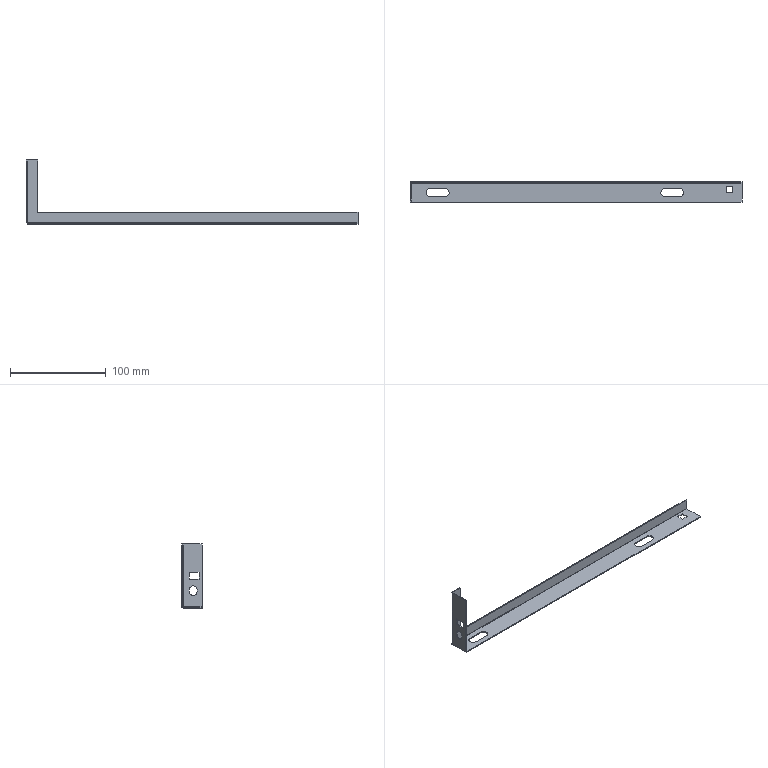Part | 1 solid | 44 faces | box 346 x 21 x 66.7 mm | volume 12385 mm3 | plane 34 | cylinder 10 | commonest cylinder face diameters 9 x4 0.4 x2 2.4 x2 8 x2
STEP:
#1=CARTESIAN_POINT('',(172.4,-1.,11.));
#2=VERTEX_POINT('',#1);
#3=CARTESIAN_POINT('',(-161.4,-1.,11.));
#4=VERTEX_POINT('',#3);
#5=CARTESIAN_POINT('',(-172.4,-1.,11.));
#6=DIRECTION('',(-1.,0.,0.));
#7=VECTOR('',#6,1000.);
#8=LINE('',#5,#7);
#9=EDGE_CURVE('',#2,#4,#8,.T.);
#10=ORIENTED_EDGE('',*,*,#9,.T.);
#11=CARTESIAN_POINT('',(-161.4,-1.,65.5));
#12=VERTEX_POINT('',#11);
#13=CARTESIAN_POINT('',(-161.4,-1.,65.5));
#14=DIRECTION('',(0.,0.,1.));
#15=VECTOR('',#14,1000.);
#16=LINE('',#13,#15);
#17=EDGE_CURVE('',#4,#12,#16,.T.);
#18=ORIENTED_EDGE('',*,*,#17,.T.);
#19=CARTESIAN_POINT('',(-172.4,-1.,65.5));
#20=VERTEX_POINT('',#19);
#21=CARTESIAN_POINT('',(-172.4,-1.,65.5));
#22=DIRECTION('',(1.,0.,0.));
#23=VECTOR('',#22,1000.);
#24=LINE('',#21,#23);
#25=EDGE_CURVE('',#20,#12,#24,.T.);
#26=ORIENTED_EDGE('',*,*,#25,.F.);
#27=CARTESIAN_POINT('',(-172.4,-1.,0.));
#28=VERTEX_POINT('',#27);
#29=CARTESIAN_POINT('',(-172.4,-1.,65.5));
#30=DIRECTION('',(0.,0.,-1.));
#31=VECTOR('',#30,1000.);
#32=LINE('',#29,#31);
#33=EDGE_CURVE('',#20,#28,#32,.T.);
#34=ORIENTED_EDGE('',*,*,#33,.T.);
#35=CARTESIAN_POINT('',(172.4,-1.,0.));
#36=VERTEX_POINT('',#35);
#37=CARTESIAN_POINT('',(-172.4,-1.,0.));
#38=DIRECTION('',(1.,0.,0.));
#39=VECTOR('',#38,1000.);
#40=LINE('',#37,#39);
#41=EDGE_CURVE('',#28,#36,#40,.T.);
#42=ORIENTED_EDGE('',*,*,#41,.T.);
#43=CARTESIAN_POINT('',(172.4,-1.,65.5));
#44=DIRECTION('',(0.,0.,-1.));
#45=VECTOR('',#44,1000.);
#46=LINE('',#43,#45);
#47=EDGE_CURVE('',#2,#36,#46,.T.);
#48=ORIENTED_EDGE('',*,*,#47,.F.);
#49=EDGE_LOOP('',(#10,#18,#26,#34,#42,#48));
#50=FACE_OUTER_BOUND('',#49,.T.);
#51=CARTESIAN_POINT('',(-172.4,-1.,65.5));
#52=DIRECTION('',(0.,1.,0.));
#53=DIRECTION('',(-1.,0.,0.));
#54=AXIS2_PLACEMENT_3D('',#51,#52,#53);
#55=PLANE('',#54);
#56=ADVANCED_FACE('',(#50),#55,.F.);
#57=CARTESIAN_POINT('',(172.4,0.,11.));
#58=VERTEX_POINT('',#57);
#59=CARTESIAN_POINT('',(172.4,-10.,11.));
#60=DIRECTION('',(0.,1.,0.));
#61=VECTOR('',#60,1000.);
#62=LINE('',#59,#61);
#63=EDGE_CURVE('',#2,#58,#62,.T.);
#64=ORIENTED_EDGE('',*,*,#63,.F.);
#65=ORIENTED_EDGE('',*,*,#47,.T.);
#66=CARTESIAN_POINT('',(172.4,0.,0.));
#67=VERTEX_POINT('',#66);
#68=CARTESIAN_POINT('',(172.4,0.,0.));
#69=DIRECTION('',(0.,-1.,0.));
#70=VECTOR('',#69,1000.);
#71=LINE('',#68,#70);
#72=EDGE_CURVE('',#67,#36,#71,.T.);
#73=ORIENTED_EDGE('',*,*,#72,.F.);
#74=CARTESIAN_POINT('',(172.4,0.,65.5));
#75=DIRECTION('',(0.,0.,-1.));
#76=VECTOR('',#75,1000.);
#77=LINE('',#74,#76);
#78=EDGE_CURVE('',#58,#67,#77,.T.);
#79=ORIENTED_EDGE('',*,*,#78,.F.);
#80=EDGE_LOOP('',(#64,#65,#73,#79));
#81=FACE_OUTER_BOUND('',#80,.T.);
#82=CARTESIAN_POINT('',(172.4,0.,65.5));
#83=DIRECTION('',(1.,0.,0.));
#84=DIRECTION('',(0.,0.,-1.));
#85=AXIS2_PLACEMENT_3D('',#82,#83,#84);
#86=PLANE('',#85);
#87=ADVANCED_FACE('',(#81),#86,.T.);
#88=CARTESIAN_POINT('',(-161.4,0.,11.));
#89=VERTEX_POINT('',#88);
#90=CARTESIAN_POINT('',(-161.4,0.,65.5));
#91=VERTEX_POINT('',#90);
#92=CARTESIAN_POINT('',(-161.4,0.,65.5));
#93=DIRECTION('',(0.,0.,1.));
#94=VECTOR('',#93,1000.);
#95=LINE('',#92,#94);
#96=EDGE_CURVE('',#89,#91,#95,.T.);
#97=ORIENTED_EDGE('',*,*,#96,.F.);
#98=CARTESIAN_POINT('',(172.4,0.,11.));
#99=DIRECTION('',(-1.,0.,0.));
#100=VECTOR('',#99,1000.);
#101=LINE('',#98,#100);
#102=EDGE_CURVE('',#58,#89,#101,.T.);
#103=ORIENTED_EDGE('',*,*,#102,.F.);
#104=ORIENTED_EDGE('',*,*,#78,.T.);
#105=CARTESIAN_POINT('',(-172.4,0.,0.));
#106=VERTEX_POINT('',#105);
#107=CARTESIAN_POINT('',(-172.4,0.,0.));
#108=DIRECTION('',(1.,0.,0.));
#109=VECTOR('',#108,1000.);
#110=LINE('',#107,#109);
#111=EDGE_CURVE('',#106,#67,#110,.T.);
#112=ORIENTED_EDGE('',*,*,#111,.F.);
#113=CARTESIAN_POINT('',(-172.4,0.,65.5));
#114=VERTEX_POINT('',#113);
#115=CARTESIAN_POINT('',(-172.4,0.,65.5));
#116=DIRECTION('',(0.,0.,-1.));
#117=VECTOR('',#116,1000.);
#118=LINE('',#115,#117);
#119=EDGE_CURVE('',#114,#106,#118,.T.);
#120=ORIENTED_EDGE('',*,*,#119,.F.);
#121=CARTESIAN_POINT('',(-172.4,0.,65.5));
#122=DIRECTION('',(1.,0.,0.));
#123=VECTOR('',#122,1000.);
#124=LINE('',#121,#123);
#125=EDGE_CURVE('',#114,#91,#124,.T.);
#126=ORIENTED_EDGE('',*,*,#125,.T.);
#127=EDGE_LOOP('',(#97,#103,#104,#112,#120,#126));
#128=FACE_OUTER_BOUND('',#127,.T.);
#129=CARTESIAN_POINT('',(-172.4,0.,65.5));
#130=DIRECTION('',(0.,1.,0.));
#131=DIRECTION('',(-1.,0.,0.));
#132=AXIS2_PLACEMENT_3D('',#129,#130,#131);
#133=PLANE('',#132);
#134=ADVANCED_FACE('',(#128),#133,.T.);
#135=ORIENTED_EDGE('',*,*,#25,.T.);
#136=CARTESIAN_POINT('',(-161.4,0.,65.5));
#137=DIRECTION('',(0.,1.,0.));
#138=VECTOR('',#137,1000.);
#139=LINE('',#136,#138);
#140=EDGE_CURVE('',#12,#91,#139,.T.);
#141=ORIENTED_EDGE('',*,*,#140,.T.);
#142=ORIENTED_EDGE('',*,*,#125,.F.);
#143=CARTESIAN_POINT('',(-172.4,-1.,65.5));
#144=DIRECTION('',(0.,1.,0.));
#145=VECTOR('',#144,1000.);
#146=LINE('',#143,#145);
#147=EDGE_CURVE('',#20,#114,#146,.T.);
#148=ORIENTED_EDGE('',*,*,#147,.F.);
#149=EDGE_LOOP('',(#135,#141,#142,#148));
#150=FACE_OUTER_BOUND('',#149,.T.);
#151=CARTESIAN_POINT('',(0.,0.,65.5));
#152=DIRECTION('',(0.,0.,-1.));
#153=DIRECTION('',(-1.,0.,0.));
#154=AXIS2_PLACEMENT_3D('',#151,#152,#153);
#155=PLANE('',#154);
#156=ADVANCED_FACE('',(#150),#155,.F.);
#157=ORIENTED_EDGE('',*,*,#63,.T.);
#158=ORIENTED_EDGE('',*,*,#102,.T.);
#159=CARTESIAN_POINT('',(-161.4,-10.,11.));
#160=DIRECTION('',(0.,1.,0.));
#161=VECTOR('',#160,1000.);
#162=LINE('',#159,#161);
#163=EDGE_CURVE('',#4,#89,#162,.T.);
#164=ORIENTED_EDGE('',*,*,#163,.F.);
#165=ORIENTED_EDGE('',*,*,#9,.F.);
#166=EDGE_LOOP('',(#157,#158,#164,#165));
#167=FACE_OUTER_BOUND('',#166,.T.);
#168=CARTESIAN_POINT('',(172.4,-10.,11.));
#169=DIRECTION('',(0.,0.,-1.));
#170=DIRECTION('',(-1.,0.,0.));
#171=AXIS2_PLACEMENT_3D('',#168,#169,#170);
#172=PLANE('',#171);
#173=ADVANCED_FACE('',(#167),#172,.F.);
#174=ORIENTED_EDGE('',*,*,#163,.T.);
#175=ORIENTED_EDGE('',*,*,#96,.T.);
#176=ORIENTED_EDGE('',*,*,#140,.F.);
#177=ORIENTED_EDGE('',*,*,#17,.F.);
#178=EDGE_LOOP('',(#174,#175,#176,#177));
#179=FACE_OUTER_BOUND('',#178,.T.);
#180=CARTESIAN_POINT('',(-161.4,-10.,65.5));
#181=DIRECTION('',(-1.,0.,0.));
#182=DIRECTION('',(0.,0.,1.));
#183=AXIS2_PLACEMENT_3D('',#180,#181,#182);
#184=PLANE('',#183);
#185=ADVANCED_FACE('',(#179),#184,.F.);
#186=CARTESIAN_POINT('',(-172.4,-1.2,-0.2));
#187=VERTEX_POINT('',#186);
#188=CARTESIAN_POINT('',(-172.4,-1.2,-1.2));
#189=VERTEX_POINT('',#188);
#190=CARTESIAN_POINT('',(-172.4,-1.2,-1.2));
#191=DIRECTION('',(0.,0.,-1.));
#192=VECTOR('',#191,1000.);
#193=LINE('',#190,#192);
#194=EDGE_CURVE('',#187,#189,#193,.T.);
#195=ORIENTED_EDGE('',*,*,#194,.F.);
#196=CARTESIAN_POINT('',(-172.4,-1.2,0.));
#197=DIRECTION('',(-1.,0.,0.));
#198=DIRECTION('',(0.,1.,0.));
#199=AXIS2_PLACEMENT_3D('',#196,#197,#198);
#200=CIRCLE('',#199,0.2);
#201=EDGE_CURVE('',#28,#187,#200,.T.);
#202=ORIENTED_EDGE('',*,*,#201,.F.);
#203=CARTESIAN_POINT('',(-172.4,-1.,0.));
#204=DIRECTION('',(0.,1.,0.));
#205=VECTOR('',#204,1000.);
#206=LINE('',#203,#205);
#207=EDGE_CURVE('',#28,#106,#206,.T.);
#208=ORIENTED_EDGE('',*,*,#207,.T.);
#209=CARTESIAN_POINT('',(-172.4,-1.2,0.));
#210=DIRECTION('',(-1.,0.,0.));
#211=DIRECTION('',(0.,1.,0.));
#212=AXIS2_PLACEMENT_3D('',#209,#210,#211);
#213=CIRCLE('',#212,1.2);
#214=EDGE_CURVE('',#106,#189,#213,.T.);
#215=ORIENTED_EDGE('',*,*,#214,.T.);
#216=EDGE_LOOP('',(#195,#202,#208,#215));
#217=FACE_OUTER_BOUND('',#216,.T.);
#218=CARTESIAN_POINT('',(-172.4,-1.2,0.));
#219=DIRECTION('',(-1.,0.,0.));
#220=DIRECTION('',(0.,-1.,0.));
#221=AXIS2_PLACEMENT_3D('',#218,#219,#220);
#222=PLANE('',#221);
#223=ADVANCED_FACE('',(#217),#222,.T.);
#224=CARTESIAN_POINT('',(172.4,-1.2,-0.2));
#225=VERTEX_POINT('',#224);
#226=CARTESIAN_POINT('',(172.4,-1.2,0.));
#227=DIRECTION('',(1.,0.,0.));
#228=DIRECTION('',(0.,1.,0.));
#229=AXIS2_PLACEMENT_3D('',#226,#227,#228);
#230=CIRCLE('',#229,0.2);
#231=EDGE_CURVE('',#225,#36,#230,.T.);
#232=ORIENTED_EDGE('',*,*,#231,.F.);
#233=CARTESIAN_POINT('',(172.4,-1.2,-1.2));
#234=VERTEX_POINT('',#233);
#235=CARTESIAN_POINT('',(172.4,-1.2,-0.2));
#236=DIRECTION('',(0.,0.,-1.));
#237=VECTOR('',#236,1000.);
#238=LINE('',#235,#237);
#239=EDGE_CURVE('',#225,#234,#238,.T.);
#240=ORIENTED_EDGE('',*,*,#239,.T.);
#241=CARTESIAN_POINT('',(172.4,-1.2,0.));
#242=DIRECTION('',(1.,0.,0.));
#243=DIRECTION('',(0.,1.,0.));
#244=AXIS2_PLACEMENT_3D('',#241,#242,#243);
#245=CIRCLE('',#244,1.2);
#246=EDGE_CURVE('',#234,#67,#245,.T.);
#247=ORIENTED_EDGE('',*,*,#246,.T.);
#248=ORIENTED_EDGE('',*,*,#72,.T.);
#249=EDGE_LOOP('',(#232,#240,#247,#248));
#250=FACE_OUTER_BOUND('',#249,.T.);
#251=CARTESIAN_POINT('',(172.4,-1.2,0.));
#252=DIRECTION('',(-1.,0.,0.));
#253=DIRECTION('',(0.,-1.,0.));
#254=AXIS2_PLACEMENT_3D('',#251,#252,#253);
#255=PLANE('',#254);
#256=ADVANCED_FACE('',(#250),#255,.F.);
#257=ORIENTED_EDGE('',*,*,#111,.T.);
#258=ORIENTED_EDGE('',*,*,#246,.F.);
#259=CARTESIAN_POINT('',(0.,-1.2,-1.2));
#260=DIRECTION('',(1.,0.,0.));
#261=VECTOR('',#260,1000.);
#262=LINE('',#259,#261);
#263=EDGE_CURVE('',#189,#234,#262,.T.);
#264=ORIENTED_EDGE('',*,*,#263,.F.);
#265=ORIENTED_EDGE('',*,*,#214,.F.);
#266=EDGE_LOOP('',(#257,#258,#264,#265));
#267=FACE_OUTER_BOUND('',#266,.T.);
#268=CARTESIAN_POINT('',(172.4,-1.2,0.));
#269=DIRECTION('',(1.,0.,0.));
#270=DIRECTION('',(0.,0.,-1.));
#271=AXIS2_PLACEMENT_3D('',#268,#269,#270);
#272=CYLINDRICAL_SURFACE('',#271,1.2);
#273=ADVANCED_FACE('',(#267),#272,.T.);
#274=ORIENTED_EDGE('',*,*,#41,.F.);
#275=ORIENTED_EDGE('',*,*,#201,.T.);
#276=CARTESIAN_POINT('',(-172.4,-1.2,-0.2));
#277=DIRECTION('',(1.,0.,0.));
#278=VECTOR('',#277,1000.);
#279=LINE('',#276,#278);
#280=EDGE_CURVE('',#187,#225,#279,.T.);
#281=ORIENTED_EDGE('',*,*,#280,.T.);
#282=ORIENTED_EDGE('',*,*,#231,.T.);
#283=EDGE_LOOP('',(#274,#275,#281,#282));
#284=FACE_OUTER_BOUND('',#283,.T.);
#285=CARTESIAN_POINT('',(172.4,-1.2,0.));
#286=DIRECTION('',(1.,0.,0.));
#287=DIRECTION('',(0.,0.,-1.));
#288=AXIS2_PLACEMENT_3D('',#285,#286,#287);
#289=CYLINDRICAL_SURFACE('',#288,0.2);
#290=ADVANCED_FACE('',(#284),#289,.F.);
#291=CARTESIAN_POINT('',(172.4,-21.,-1.2));
#292=VERTEX_POINT('',#291);
#293=CARTESIAN_POINT('',(172.4,-1.,-1.2));
#294=DIRECTION('',(0.,1.,0.));
#295=VECTOR('',#294,1000.);
#296=LINE('',#293,#295);
#297=EDGE_CURVE('',#292,#234,#296,.T.);
#298=ORIENTED_EDGE('',*,*,#297,.T.);
#299=ORIENTED_EDGE('',*,*,#239,.F.);
#300=CARTESIAN_POINT('',(172.4,-21.,-0.2));
#301=VERTEX_POINT('',#300);
#302=CARTESIAN_POINT('',(172.4,0.,-0.2));
#303=DIRECTION('',(0.,1.,0.));
#304=VECTOR('',#303,1000.);
#305=LINE('',#302,#304);
#306=EDGE_CURVE('',#301,#225,#305,.T.);
#307=ORIENTED_EDGE('',*,*,#306,.F.);
#308=CARTESIAN_POINT('',(172.4,-21.,-1.2));
#309=DIRECTION('',(0.,0.,1.));
#310=VECTOR('',#309,1000.);
#311=LINE('',#308,#310);
#312=EDGE_CURVE('',#292,#301,#311,.T.);
#313=ORIENTED_EDGE('',*,*,#312,.F.);
#314=EDGE_LOOP('',(#298,#299,#307,#313));
#315=FACE_OUTER_BOUND('',#314,.T.);
#316=CARTESIAN_POINT('',(172.4,-1.,-1.2));
#317=DIRECTION('',(1.,0.,0.));
#318=DIRECTION('',(0.,0.,-1.));
#319=AXIS2_PLACEMENT_3D('',#316,#317,#318);
#320=PLANE('',#319);
#321=ADVANCED_FACE('',(#315),#320,.T.);
#322=CARTESIAN_POINT('',(-172.4,-21.,-0.2));
#323=VERTEX_POINT('',#322);
#324=CARTESIAN_POINT('',(-172.4,0.,-0.2));
#325=DIRECTION('',(0.,-1.,0.));
#326=VECTOR('',#325,1000.);
#327=LINE('',#324,#326);
#328=EDGE_CURVE('',#187,#323,#327,.T.);
#329=ORIENTED_EDGE('',*,*,#328,.F.);
#330=ORIENTED_EDGE('',*,*,#194,.T.);
#331=CARTESIAN_POINT('',(-172.4,-21.,-1.2));
#332=VERTEX_POINT('',#331);
#333=CARTESIAN_POINT('',(-172.4,-21.,-1.2));
#334=DIRECTION('',(0.,-1.,0.));
#335=VECTOR('',#334,1000.);
#336=LINE('',#333,#335);
#337=EDGE_CURVE('',#189,#332,#336,.T.);
#338=ORIENTED_EDGE('',*,*,#337,.T.);
#339=CARTESIAN_POINT('',(-172.4,-21.,-1.2));
#340=DIRECTION('',(0.,0.,1.));
#341=VECTOR('',#340,1000.);
#342=LINE('',#339,#341);
#343=EDGE_CURVE('',#332,#323,#342,.T.);
#344=ORIENTED_EDGE('',*,*,#343,.T.);
#345=EDGE_LOOP('',(#329,#330,#338,#344));
#346=FACE_OUTER_BOUND('',#345,.T.);
#347=CARTESIAN_POINT('',(-172.4,-21.,-1.2));
#348=DIRECTION('',(-1.,0.,0.));
#349=DIRECTION('',(0.,0.,1.));
#350=AXIS2_PLACEMENT_3D('',#347,#348,#349);
#351=PLANE('',#350);
#352=ADVANCED_FACE('',(#346),#351,.T.);
#353=CARTESIAN_POINT('',(162.9,-4.3,-1.2));
#354=VERTEX_POINT('',#353);
#355=CARTESIAN_POINT('',(162.9,-11.3,-1.2));
#356=VERTEX_POINT('',#355);
#357=CARTESIAN_POINT('',(162.9,-11.3,-1.2));
#358=DIRECTION('',(0.,-1.,0.));
#359=VECTOR('',#358,1000.);
#360=LINE('',#357,#359);
#361=EDGE_CURVE('',#354,#356,#360,.T.);
#362=ORIENTED_EDGE('',*,*,#361,.F.);
#363=CARTESIAN_POINT('',(155.9,-4.3,-1.2));
#364=VERTEX_POINT('',#363);
#365=CARTESIAN_POINT('',(162.9,-4.3,-1.2));
#366=DIRECTION('',(1.,0.,0.));
#367=VECTOR('',#366,1000.);
#368=LINE('',#365,#367);
#369=EDGE_CURVE('',#364,#354,#368,.T.);
#370=ORIENTED_EDGE('',*,*,#369,.F.);
#371=CARTESIAN_POINT('',(155.9,-11.3,-1.2));
#372=VERTEX_POINT('',#371);
#373=CARTESIAN_POINT('',(155.9,-11.3,-1.2));
#374=DIRECTION('',(0.,1.,0.));
#375=VECTOR('',#374,1000.);
#376=LINE('',#373,#375);
#377=EDGE_CURVE('',#372,#364,#376,.T.);
#378=ORIENTED_EDGE('',*,*,#377,.F.);
#379=CARTESIAN_POINT('',(162.9,-11.3,-1.2));
#380=DIRECTION('',(-1.,0.,0.));
#381=VECTOR('',#380,1000.);
#382=LINE('',#379,#381);
#383=EDGE_CURVE('',#356,#372,#382,.T.);
#384=ORIENTED_EDGE('',*,*,#383,.F.);
#385=EDGE_LOOP('',(#362,#370,#378,#384));
#386=FACE_BOUND('',#385,.T.);
#387=CARTESIAN_POINT('',(-152.3,-15.5,-1.2));
#388=VERTEX_POINT('',#387);
#389=CARTESIAN_POINT('',(-152.3,-6.5,-1.2));
#390=VERTEX_POINT('',#389);
#391=CARTESIAN_POINT('',(-152.3,-11.,-1.2));
#392=DIRECTION('',(0.,0.,-1.));
#393=DIRECTION('',(0.,1.,0.));
#394=AXIS2_PLACEMENT_3D('',#391,#392,#393);
#395=CIRCLE('',#394,4.5);
#396=EDGE_CURVE('',#388,#390,#395,.T.);
#397=ORIENTED_EDGE('',*,*,#396,.F.);
#398=CARTESIAN_POINT('',(-137.3,-15.5,-1.2));
#399=VERTEX_POINT('',#398);
#400=CARTESIAN_POINT('',(-152.3,-15.5,-1.2));
#401=DIRECTION('',(-1.,0.,0.));
#402=VECTOR('',#401,1000.);
#403=LINE('',#400,#402);
#404=EDGE_CURVE('',#399,#388,#403,.T.);
#405=ORIENTED_EDGE('',*,*,#404,.F.);
#406=CARTESIAN_POINT('',(-137.3,-6.5,-1.2));
#407=VERTEX_POINT('',#406);
#408=CARTESIAN_POINT('',(-137.3,-11.,-1.2));
#409=DIRECTION('',(0.,0.,-1.));
#410=DIRECTION('',(0.,1.,0.));
#411=AXIS2_PLACEMENT_3D('',#408,#409,#410);
#412=CIRCLE('',#411,4.5);
#413=EDGE_CURVE('',#407,#399,#412,.T.);
#414=ORIENTED_EDGE('',*,*,#413,.F.);
#415=CARTESIAN_POINT('',(-152.3,-6.5,-1.2));
#416=DIRECTION('',(1.,0.,0.));
#417=VECTOR('',#416,1000.);
#418=LINE('',#415,#417);
#419=EDGE_CURVE('',#390,#407,#418,.T.);
#420=ORIENTED_EDGE('',*,*,#419,.F.);
#421=EDGE_LOOP('',(#397,#405,#414,#420));
#422=FACE_BOUND('',#421,.T.);
#423=CARTESIAN_POINT('',(92.2,-15.5,-1.2));
#424=VERTEX_POINT('',#423);
#425=CARTESIAN_POINT('',(92.2,-6.5,-1.2));
#426=VERTEX_POINT('',#425);
#427=CARTESIAN_POINT('',(92.2,-11.,-1.2));
#428=DIRECTION('',(0.,0.,-1.));
#429=DIRECTION('',(0.,1.,0.));
#430=AXIS2_PLACEMENT_3D('',#427,#428,#429);
#431=CIRCLE('',#430,4.5);
#432=EDGE_CURVE('',#424,#426,#431,.T.);
#433=ORIENTED_EDGE('',*,*,#432,.F.);
#434=CARTESIAN_POINT('',(107.2,-15.5,-1.2));
#435=VERTEX_POINT('',#434);
#436=CARTESIAN_POINT('',(92.2,-15.5,-1.2));
#437=DIRECTION('',(-1.,0.,0.));
#438=VECTOR('',#437,1000.);
#439=LINE('',#436,#438);
#440=EDGE_CURVE('',#435,#424,#439,.T.);
#441=ORIENTED_EDGE('',*,*,#440,.F.);
#442=CARTESIAN_POINT('',(107.2,-6.5,-1.2));
#443=VERTEX_POINT('',#442);
#444=CARTESIAN_POINT('',(107.2,-11.,-1.2));
#445=DIRECTION('',(0.,0.,-1.));
#446=DIRECTION('',(0.,1.,0.));
#447=AXIS2_PLACEMENT_3D('',#444,#445,#446);
#448=CIRCLE('',#447,4.5);
#449=EDGE_CURVE('',#443,#435,#448,.T.);
#450=ORIENTED_EDGE('',*,*,#449,.F.);
#451=CARTESIAN_POINT('',(92.2,-6.5,-1.2));
#452=DIRECTION('',(1.,0.,0.));
#453=VECTOR('',#452,1000.);
#454=LINE('',#451,#453);
#455=EDGE_CURVE('',#426,#443,#454,.T.);
#456=ORIENTED_EDGE('',*,*,#455,.F.);
#457=EDGE_LOOP('',(#433,#441,#450,#456));
#458=FACE_BOUND('',#457,.T.);
#459=ORIENTED_EDGE('',*,*,#337,.F.);
#460=ORIENTED_EDGE('',*,*,#263,.T.);
#461=ORIENTED_EDGE('',*,*,#297,.F.);
#462=CARTESIAN_POINT('',(172.4,-21.,-1.2));
#463=DIRECTION('',(1.,0.,0.));
#464=VECTOR('',#463,1000.);
#465=LINE('',#462,#464);
#466=EDGE_CURVE('',#332,#292,#465,.T.);
#467=ORIENTED_EDGE('',*,*,#466,.F.);
#468=EDGE_LOOP('',(#459,#460,#461,#467));
#469=FACE_OUTER_BOUND('',#468,.T.);
#470=CARTESIAN_POINT('',(0.,0.,-1.2));
#471=DIRECTION('',(0.,0.,-1.));
#472=DIRECTION('',(0.,1.,0.));
#473=AXIS2_PLACEMENT_3D('',#470,#471,#472);
#474=PLANE('',#473);
#475=ADVANCED_FACE('',(#386,#422,#458,#469),#474,.T.);
#476=CARTESIAN_POINT('',(155.9,-4.3,-0.2));
#477=VERTEX_POINT('',#476);
#478=CARTESIAN_POINT('',(162.9,-4.3,-0.2));
#479=VERTEX_POINT('',#478);
#480=CARTESIAN_POINT('',(0.,-4.3,-0.2));
#481=DIRECTION('',(1.,0.,0.));
#482=VECTOR('',#481,1000.);
#483=LINE('',#480,#482);
#484=EDGE_CURVE('',#477,#479,#483,.T.);
#485=ORIENTED_EDGE('',*,*,#484,.T.);
#486=CARTESIAN_POINT('',(162.9,-11.3,-0.2));
#487=VERTEX_POINT('',#486);
#488=CARTESIAN_POINT('',(162.9,0.,-0.2));
#489=DIRECTION('',(0.,-1.,0.));
#490=VECTOR('',#489,1000.);
#491=LINE('',#488,#490);
#492=EDGE_CURVE('',#479,#487,#491,.T.);
#493=ORIENTED_EDGE('',*,*,#492,.T.);
#494=CARTESIAN_POINT('',(155.9,-11.3,-0.2));
#495=VERTEX_POINT('',#494);
#496=CARTESIAN_POINT('',(0.,-11.3,-0.2));
#497=DIRECTION('',(-1.,0.,0.));
#498=VECTOR('',#497,1000.);
#499=LINE('',#496,#498);
#500=EDGE_CURVE('',#487,#495,#499,.T.);
#501=ORIENTED_EDGE('',*,*,#500,.T.);
#502=CARTESIAN_POINT('',(155.9,0.,-0.2));
#503=DIRECTION('',(0.,1.,0.));
#504=VECTOR('',#503,1000.);
#505=LINE('',#502,#504);
#506=EDGE_CURVE('',#495,#477,#505,.T.);
#507=ORIENTED_EDGE('',*,*,#506,.T.);
#508=EDGE_LOOP('',(#485,#493,#501,#507));
#509=FACE_BOUND('',#508,.T.);
#510=CARTESIAN_POINT('',(-137.3,-15.5,-0.2));
#511=VERTEX_POINT('',#510);
#512=CARTESIAN_POINT('',(-152.3,-15.5,-0.2));
#513=VERTEX_POINT('',#512);
#514=CARTESIAN_POINT('',(0.,-15.5,-0.2));
#515=DIRECTION('',(-1.,0.,0.));
#516=VECTOR('',#515,1000.);
#517=LINE('',#514,#516);
#518=EDGE_CURVE('',#511,#513,#517,.T.);
#519=ORIENTED_EDGE('',*,*,#518,.T.);
#520=CARTESIAN_POINT('',(-152.3,-6.5,-0.2));
#521=VERTEX_POINT('',#520);
#522=CARTESIAN_POINT('',(-152.3,-11.,-0.2));
#523=DIRECTION('',(0.,0.,-1.));
#524=DIRECTION('',(0.,1.,0.));
#525=AXIS2_PLACEMENT_3D('',#522,#523,#524);
#526=CIRCLE('',#525,4.5);
#527=EDGE_CURVE('',#513,#521,#526,.T.);
#528=ORIENTED_EDGE('',*,*,#527,.T.);
#529=CARTESIAN_POINT('',(-137.3,-6.5,-0.2));
#530=VERTEX_POINT('',#529);
#531=CARTESIAN_POINT('',(0.,-6.5,-0.2));
#532=DIRECTION('',(1.,0.,0.));
#533=VECTOR('',#532,1000.);
#534=LINE('',#531,#533);
#535=EDGE_CURVE('',#521,#530,#534,.T.);
#536=ORIENTED_EDGE('',*,*,#535,.T.);
#537=CARTESIAN_POINT('',(-137.3,-11.,-0.2));
#538=DIRECTION('',(0.,0.,-1.));
#539=DIRECTION('',(0.,1.,0.));
#540=AXIS2_PLACEMENT_3D('',#537,#538,#539);
#541=CIRCLE('',#540,4.5);
#542=EDGE_CURVE('',#530,#511,#541,.T.);
#543=ORIENTED_EDGE('',*,*,#542,.T.);
#544=EDGE_LOOP('',(#519,#528,#536,#543));
#545=FACE_BOUND('',#544,.T.);
#546=CARTESIAN_POINT('',(107.2,-15.5,-0.2));
#547=VERTEX_POINT('',#546);
#548=CARTESIAN_POINT('',(92.2,-15.5,-0.2));
#549=VERTEX_POINT('',#548);
#550=CARTESIAN_POINT('',(0.,-15.5,-0.2));
#551=DIRECTION('',(-1.,0.,0.));
#552=VECTOR('',#551,1000.);
#553=LINE('',#550,#552);
#554=EDGE_CURVE('',#547,#549,#553,.T.);
#555=ORIENTED_EDGE('',*,*,#554,.T.);
#556=CARTESIAN_POINT('',(92.2,-6.5,-0.2));
#557=VERTEX_POINT('',#556);
#558=CARTESIAN_POINT('',(92.2,-11.,-0.2));
#559=DIRECTION('',(0.,0.,-1.));
#560=DIRECTION('',(0.,1.,0.));
#561=AXIS2_PLACEMENT_3D('',#558,#559,#560);
#562=CIRCLE('',#561,4.5);
#563=EDGE_CURVE('',#549,#557,#562,.T.);
#564=ORIENTED_EDGE('',*,*,#563,.T.);
#565=CARTESIAN_POINT('',(107.2,-6.5,-0.2));
#566=VERTEX_POINT('',#565);
#567=CARTESIAN_POINT('',(0.,-6.5,-0.2));
#568=DIRECTION('',(1.,0.,0.));
#569=VECTOR('',#568,1000.);
#570=LINE('',#567,#569);
#571=EDGE_CURVE('',#557,#566,#570,.T.);
#572=ORIENTED_EDGE('',*,*,#571,.T.);
#573=CARTESIAN_POINT('',(107.2,-11.,-0.2));
#574=DIRECTION('',(0.,0.,-1.));
#575=DIRECTION('',(0.,1.,0.));
#576=AXIS2_PLACEMENT_3D('',#573,#574,#575);
#577=CIRCLE('',#576,4.5);
#578=EDGE_CURVE('',#566,#547,#577,.T.);
#579=ORIENTED_EDGE('',*,*,#578,.T.);
#580=EDGE_LOOP('',(#555,#564,#572,#579));
#581=FACE_BOUND('',#580,.T.);
#582=ORIENTED_EDGE('',*,*,#280,.F.);
#583=ORIENTED_EDGE('',*,*,#328,.T.);
#584=CARTESIAN_POINT('',(0.,-21.,-0.2));
#585=DIRECTION('',(1.,0.,0.));
#586=VECTOR('',#585,1000.);
#587=LINE('',#584,#586);
#588=EDGE_CURVE('',#323,#301,#587,.T.);
#589=ORIENTED_EDGE('',*,*,#588,.T.);
#590=ORIENTED_EDGE('',*,*,#306,.T.);
#591=EDGE_LOOP('',(#582,#583,#589,#590));
#592=FACE_OUTER_BOUND('',#591,.T.);
#593=CARTESIAN_POINT('',(0.,0.,-0.2));
#594=DIRECTION('',(0.,0.,-1.));
#595=DIRECTION('',(0.,1.,0.));
#596=AXIS2_PLACEMENT_3D('',#593,#594,#595);
#597=PLANE('',#596);
#598=ADVANCED_FACE('',(#509,#545,#581,#592),#597,.F.);
#599=ORIENTED_EDGE('',*,*,#588,.F.);
#600=ORIENTED_EDGE('',*,*,#343,.F.);
#601=ORIENTED_EDGE('',*,*,#466,.T.);
#602=ORIENTED_EDGE('',*,*,#312,.T.);
#603=EDGE_LOOP('',(#599,#600,#601,#602));
#604=FACE_OUTER_BOUND('',#603,.T.);
#605=CARTESIAN_POINT('',(172.4,-21.,-1.2));
#606=DIRECTION('',(0.,-1.,0.));
#607=DIRECTION('',(0.,0.,-1.));
#608=AXIS2_PLACEMENT_3D('',#605,#606,#607);
#609=PLANE('',#608);
#610=ADVANCED_FACE('',(#604),#609,.T.);
#611=CARTESIAN_POINT('',(-172.6,-1.2,65.5));
#612=VERTEX_POINT('',#611);
#613=CARTESIAN_POINT('',(-173.6,-1.2,65.5));
#614=VERTEX_POINT('',#613);
#615=CARTESIAN_POINT('',(-173.6,-1.2,65.5));
#616=DIRECTION('',(-1.,0.,0.));
#617=VECTOR('',#616,1000.);
#618=LINE('',#615,#617);
#619=EDGE_CURVE('',#612,#614,#618,.T.);
#620=ORIENTED_EDGE('',*,*,#619,.F.);
#621=CARTESIAN_POINT('',(-172.4,-1.2,65.5));
#622=DIRECTION('',(0.,0.,1.));
#623=DIRECTION('',(-1.,0.,0.));
#624=AXIS2_PLACEMENT_3D('',#621,#622,#623);
#625=CIRCLE('',#624,0.2);
#626=EDGE_CURVE('',#20,#612,#625,.T.);
#627=ORIENTED_EDGE('',*,*,#626,.F.);
#628=ORIENTED_EDGE('',*,*,#147,.T.);
#629=CARTESIAN_POINT('',(-172.4,-1.2,65.5));
#630=DIRECTION('',(0.,0.,1.));
#631=DIRECTION('',(-1.,0.,0.));
#632=AXIS2_PLACEMENT_3D('',#629,#630,#631);
#633=CIRCLE('',#632,1.2);
#634=EDGE_CURVE('',#114,#614,#633,.T.);
#635=ORIENTED_EDGE('',*,*,#634,.T.);
#636=EDGE_LOOP('',(#620,#627,#628,#635));
#637=FACE_OUTER_BOUND('',#636,.T.);
#638=CARTESIAN_POINT('',(-172.4,-1.2,65.5));
#639=DIRECTION('',(0.,0.,1.));
#640=DIRECTION('',(1.,0.,0.));
#641=AXIS2_PLACEMENT_3D('',#638,#639,#640);
#642=PLANE('',#641);
#643=ADVANCED_FACE('',(#637),#642,.T.);
#644=CARTESIAN_POINT('',(-172.6,-1.2,0.));
#645=VERTEX_POINT('',#644);
#646=CARTESIAN_POINT('',(-172.4,-1.2,0.));
#647=DIRECTION('',(0.,0.,-1.));
#648=DIRECTION('',(-1.,0.,0.));
#649=AXIS2_PLACEMENT_3D('',#646,#647,#648);
#650=CIRCLE('',#649,0.2);
#651=EDGE_CURVE('',#645,#28,#650,.T.);
#652=ORIENTED_EDGE('',*,*,#651,.F.);
#653=CARTESIAN_POINT('',(-173.6,-1.2,0.));
#654=VERTEX_POINT('',#653);
#655=CARTESIAN_POINT('',(-172.6,-1.2,0.));
#656=DIRECTION('',(-1.,0.,0.));
#657=VECTOR('',#656,1000.);
#658=LINE('',#655,#657);
#659=EDGE_CURVE('',#645,#654,#658,.T.);
#660=ORIENTED_EDGE('',*,*,#659,.T.);
#661=CARTESIAN_POINT('',(-172.4,-1.2,0.));
#662=DIRECTION('',(0.,0.,-1.));
#663=DIRECTION('',(-1.,0.,0.));
#664=AXIS2_PLACEMENT_3D('',#661,#662,#663);
#665=CIRCLE('',#664,1.2);
#666=EDGE_CURVE('',#654,#106,#665,.T.);
#667=ORIENTED_EDGE('',*,*,#666,.T.);
#668=ORIENTED_EDGE('',*,*,#207,.F.);
#669=EDGE_LOOP('',(#652,#660,#667,#668));
#670=FACE_OUTER_BOUND('',#669,.T.);
#671=CARTESIAN_POINT('',(-172.4,-1.2,0.));
#672=DIRECTION('',(0.,0.,1.));
#673=DIRECTION('',(1.,0.,0.));
#674=AXIS2_PLACEMENT_3D('',#671,#672,#673);
#675=PLANE('',#674);
#676=ADVANCED_FACE('',(#670),#675,.F.);
#677=ORIENTED_EDGE('',*,*,#119,.T.);
#678=ORIENTED_EDGE('',*,*,#666,.F.);
#679=CARTESIAN_POINT('',(-173.6,-1.2,0.));
#680=DIRECTION('',(0.,0.,-1.));
#681=VECTOR('',#680,1000.);
#682=LINE('',#679,#681);
#683=EDGE_CURVE('',#614,#654,#682,.T.);
#684=ORIENTED_EDGE('',*,*,#683,.F.);
#685=ORIENTED_EDGE('',*,*,#634,.F.);
#686=EDGE_LOOP('',(#677,#678,#684,#685));
#687=FACE_OUTER_BOUND('',#686,.T.);
#688=CARTESIAN_POINT('',(-172.4,-1.2,0.));
#689=DIRECTION('',(0.,0.,-1.));
#690=DIRECTION('',(-1.,0.,0.));
#691=AXIS2_PLACEMENT_3D('',#688,#689,#690);
#692=CYLINDRICAL_SURFACE('',#691,1.2);
#693=ADVANCED_FACE('',(#687),#692,.T.);
#694=ORIENTED_EDGE('',*,*,#33,.F.);
#695=ORIENTED_EDGE('',*,*,#626,.T.);
#696=CARTESIAN_POINT('',(-172.6,-1.2,65.5));
#697=DIRECTION('',(0.,0.,-1.));
#698=VECTOR('',#697,1000.);
#699=LINE('',#696,#698);
#700=EDGE_CURVE('',#612,#645,#699,.T.);
#701=ORIENTED_EDGE('',*,*,#700,.T.);
#702=ORIENTED_EDGE('',*,*,#651,.T.);
#703=EDGE_LOOP('',(#694,#695,#701,#702));
#704=FACE_OUTER_BOUND('',#703,.T.);
#705=CARTESIAN_POINT('',(-172.4,-1.2,0.));
#706=DIRECTION('',(0.,0.,-1.));
#707=DIRECTION('',(-1.,0.,0.));
#708=AXIS2_PLACEMENT_3D('',#705,#706,#707);
#709=CYLINDRICAL_SURFACE('',#708,0.2);
#710=ADVANCED_FACE('',(#704),#709,.F.);
#711=CARTESIAN_POINT('',(-173.6,-21.,0.));
#712=VERTEX_POINT('',#711);
#713=CARTESIAN_POINT('',(-173.6,-1.,0.));
#714=DIRECTION('',(0.,1.,0.));
#715=VECTOR('',#714,1000.);
#716=LINE('',#713,#715);
#717=EDGE_CURVE('',#712,#654,#716,.T.);
#718=ORIENTED_EDGE('',*,*,#717,.T.);
#719=ORIENTED_EDGE('',*,*,#659,.F.);
#720=CARTESIAN_POINT('',(-172.6,-21.,0.));
#721=VERTEX_POINT('',#720);
#722=CARTESIAN_POINT('',(-172.6,0.,0.));
#723=DIRECTION('',(0.,1.,0.));
#724=VECTOR('',#723,1000.);
#725=LINE('',#722,#724);
#726=EDGE_CURVE('',#721,#645,#725,.T.);
#727=ORIENTED_EDGE('',*,*,#726,.F.);
#728=CARTESIAN_POINT('',(-173.6,-21.,0.));
#729=DIRECTION('',(1.,0.,0.));
#730=VECTOR('',#729,1000.);
#731=LINE('',#728,#730);
#732=EDGE_CURVE('',#712,#721,#731,.T.);
#733=ORIENTED_EDGE('',*,*,#732,.F.);
#734=EDGE_LOOP('',(#718,#719,#727,#733));
#735=FACE_OUTER_BOUND('',#734,.T.);
#736=CARTESIAN_POINT('',(-173.6,-1.,0.));
#737=DIRECTION('',(0.,0.,-1.));
#738=DIRECTION('',(-1.,0.,0.));
#739=AXIS2_PLACEMENT_3D('',#736,#737,#738);
#740=PLANE('',#739);
#741=ADVANCED_FACE('',(#735),#740,.T.);
#742=CARTESIAN_POINT('',(-172.6,-21.,65.5));
#743=VERTEX_POINT('',#742);
#744=CARTESIAN_POINT('',(-172.6,0.,65.5));
#745=DIRECTION('',(0.,-1.,0.));
#746=VECTOR('',#745,1000.);
#747=LINE('',#744,#746);
#748=EDGE_CURVE('',#612,#743,#747,.T.);
#749=ORIENTED_EDGE('',*,*,#748,.F.);
#750=ORIENTED_EDGE('',*,*,#619,.T.);
#751=CARTESIAN_POINT('',(-173.6,-21.,65.5));
#752=VERTEX_POINT('',#751);
#753=CARTESIAN_POINT('',(-173.6,-21.,65.5));
#754=DIRECTION('',(0.,-1.,0.));
#755=VECTOR('',#754,1000.);
#756=LINE('',#753,#755);
#757=EDGE_CURVE('',#614,#752,#756,.T.);
#758=ORIENTED_EDGE('',*,*,#757,.T.);
#759=CARTESIAN_POINT('',(-173.6,-21.,65.5));
#760=DIRECTION('',(1.,0.,0.));
#761=VECTOR('',#760,1000.);
#762=LINE('',#759,#761);
#763=EDGE_CURVE('',#752,#743,#762,.T.);
#764=ORIENTED_EDGE('',*,*,#763,.T.);
#765=EDGE_LOOP('',(#749,#750,#758,#764));
#766=FACE_OUTER_BOUND('',#765,.T.);
#767=CARTESIAN_POINT('',(-173.6,-21.,65.5));
#768=DIRECTION('',(0.,0.,1.));
#769=DIRECTION('',(1.,0.,0.));
#770=AXIS2_PLACEMENT_3D('',#767,#768,#769);
#771=PLANE('',#770);
#772=ADVANCED_FACE('',(#766),#771,.T.);
#773=CARTESIAN_POINT('',(-173.6,-7.8,28.8));
#774=VERTEX_POINT('',#773);
#775=CARTESIAN_POINT('',(-173.6,-17.8,28.8));
#776=VERTEX_POINT('',#775);
#777=CARTESIAN_POINT('',(-173.6,-17.8,28.8));
#778=DIRECTION('',(0.,-1.,0.));
#779=VECTOR('',#778,1000.);
#780=LINE('',#777,#779);
#781=EDGE_CURVE('',#774,#776,#780,.T.);
#782=ORIENTED_EDGE('',*,*,#781,.F.);
#783=CARTESIAN_POINT('',(-173.6,-7.8,35.8));
#784=VERTEX_POINT('',#783);
#785=CARTESIAN_POINT('',(-173.6,-7.8,35.8));
#786=DIRECTION('',(0.,0.,-1.));
#787=VECTOR('',#786,1000.);
#788=LINE('',#785,#787);
#789=EDGE_CURVE('',#784,#774,#788,.T.);
#790=ORIENTED_EDGE('',*,*,#789,.F.);
#791=CARTESIAN_POINT('',(-173.6,-17.8,35.8));
#792=VERTEX_POINT('',#791);
#793=CARTESIAN_POINT('',(-173.6,-17.8,35.8));
#794=DIRECTION('',(0.,1.,0.));
#795=VECTOR('',#794,1000.);
#796=LINE('',#793,#795);
#797=EDGE_CURVE('',#792,#784,#796,.T.);
#798=ORIENTED_EDGE('',*,*,#797,.F.);
#799=CARTESIAN_POINT('',(-173.6,-17.8,35.8));
#800=DIRECTION('',(0.,0.,1.));
#801=VECTOR('',#800,1000.);
#802=LINE('',#799,#801);
#803=EDGE_CURVE('',#776,#792,#802,.T.);
#804=ORIENTED_EDGE('',*,*,#803,.F.);
#805=EDGE_LOOP('',(#782,#790,#798,#804));
#806=FACE_BOUND('',#805,.T.);
#807=CARTESIAN_POINT('',(-173.6,-7.8,15.8));
#808=VERTEX_POINT('',#807);
#809=CARTESIAN_POINT('',(-173.6,-15.8,15.8));
#810=VERTEX_POINT('',#809);
#811=CARTESIAN_POINT('',(-173.6,-11.8,15.8));
#812=DIRECTION('',(-1.,0.,0.));
#813=DIRECTION('',(0.,-1.,0.));
#814=AXIS2_PLACEMENT_3D('',#811,#812,#813);
#815=CIRCLE('',#814,4.);
#816=EDGE_CURVE('',#808,#810,#815,.T.);
#817=ORIENTED_EDGE('',*,*,#816,.F.);
#818=CARTESIAN_POINT('',(-173.6,-7.8,17.8));
#819=VERTEX_POINT('',#818);
#820=CARTESIAN_POINT('',(-173.6,-7.8,15.8));
#821=DIRECTION('',(0.,0.,-1.));
#822=VECTOR('',#821,1000.);
#823=LINE('',#820,#822);
#824=EDGE_CURVE('',#819,#808,#823,.T.);
#825=ORIENTED_EDGE('',*,*,#824,.F.);
#826=CARTESIAN_POINT('',(-173.6,-15.8,17.8));
#827=VERTEX_POINT('',#826);
#828=CARTESIAN_POINT('',(-173.6,-11.8,17.8));
#829=DIRECTION('',(-1.,0.,0.));
#830=DIRECTION('',(0.,-1.,0.));
#831=AXIS2_PLACEMENT_3D('',#828,#829,#830);
#832=CIRCLE('',#831,4.);
#833=EDGE_CURVE('',#827,#819,#832,.T.);
#834=ORIENTED_EDGE('',*,*,#833,.F.);
#835=CARTESIAN_POINT('',(-173.6,-15.8,15.8));
#836=DIRECTION('',(0.,0.,1.));
#837=VECTOR('',#836,1000.);
#838=LINE('',#835,#837);
#839=EDGE_CURVE('',#810,#827,#838,.T.);
#840=ORIENTED_EDGE('',*,*,#839,.F.);
#841=EDGE_LOOP('',(#817,#825,#834,#840));
#842=FACE_BOUND('',#841,.T.);
#843=ORIENTED_EDGE('',*,*,#757,.F.);
#844=ORIENTED_EDGE('',*,*,#683,.T.);
#845=ORIENTED_EDGE('',*,*,#717,.F.);
#846=CARTESIAN_POINT('',(-173.6,-21.,0.));
#847=DIRECTION('',(0.,0.,-1.));
#848=VECTOR('',#847,1000.);
#849=LINE('',#846,#848);
#850=EDGE_CURVE('',#752,#712,#849,.T.);
#851=ORIENTED_EDGE('',*,*,#850,.F.);
#852=EDGE_LOOP('',(#843,#844,#845,#851));
#853=FACE_OUTER_BOUND('',#852,.T.);
#854=CARTESIAN_POINT('',(-173.6,0.,0.));
#855=DIRECTION('',(-1.,0.,0.));
#856=DIRECTION('',(0.,-1.,0.));
#857=AXIS2_PLACEMENT_3D('',#854,#855,#856);
#858=PLANE('',#857);
#859=ADVANCED_FACE('',(#806,#842,#853),#858,.T.);
#860=CARTESIAN_POINT('',(-172.6,-7.8,35.8));
#861=VERTEX_POINT('',#860);
#862=CARTESIAN_POINT('',(-172.6,-7.8,28.8));
#863=VERTEX_POINT('',#862);
#864=CARTESIAN_POINT('',(-172.6,-7.8,0.));
#865=DIRECTION('',(0.,0.,-1.));
#866=VECTOR('',#865,1000.);
#867=LINE('',#864,#866);
#868=EDGE_CURVE('',#861,#863,#867,.T.);
#869=ORIENTED_EDGE('',*,*,#868,.T.);
#870=CARTESIAN_POINT('',(-172.6,-17.8,28.8));
#871=VERTEX_POINT('',#870);
#872=CARTESIAN_POINT('',(-172.6,0.,28.8));
#873=DIRECTION('',(0.,-1.,0.));
#874=VECTOR('',#873,1000.);
#875=LINE('',#872,#874);
#876=EDGE_CURVE('',#863,#871,#875,.T.);
#877=ORIENTED_EDGE('',*,*,#876,.T.);
#878=CARTESIAN_POINT('',(-172.6,-17.8,35.8));
#879=VERTEX_POINT('',#878);
#880=CARTESIAN_POINT('',(-172.6,-17.8,0.));
#881=DIRECTION('',(0.,0.,1.));
#882=VECTOR('',#881,1000.);
#883=LINE('',#880,#882);
#884=EDGE_CURVE('',#871,#879,#883,.T.);
#885=ORIENTED_EDGE('',*,*,#884,.T.);
#886=CARTESIAN_POINT('',(-172.6,0.,35.8));
#887=DIRECTION('',(0.,1.,0.));
#888=VECTOR('',#887,1000.);
#889=LINE('',#886,#888);
#890=EDGE_CURVE('',#879,#861,#889,.T.);
#891=ORIENTED_EDGE('',*,*,#890,.T.);
#892=EDGE_LOOP('',(#869,#877,#885,#891));
#893=FACE_BOUND('',#892,.T.);
#894=CARTESIAN_POINT('',(-172.6,-7.8,17.8));
#895=VERTEX_POINT('',#894);
#896=CARTESIAN_POINT('',(-172.6,-7.8,15.8));
#897=VERTEX_POINT('',#896);
#898=CARTESIAN_POINT('',(-172.6,-7.8,0.));
#899=DIRECTION('',(0.,0.,-1.));
#900=VECTOR('',#899,1000.);
#901=LINE('',#898,#900);
#902=EDGE_CURVE('',#895,#897,#901,.T.);
#903=ORIENTED_EDGE('',*,*,#902,.T.);
#904=CARTESIAN_POINT('',(-172.6,-15.8,15.8));
#905=VERTEX_POINT('',#904);
#906=CARTESIAN_POINT('',(-172.6,-11.8,15.8));
#907=DIRECTION('',(-1.,0.,0.));
#908=DIRECTION('',(0.,-1.,0.));
#909=AXIS2_PLACEMENT_3D('',#906,#907,#908);
#910=CIRCLE('',#909,4.);
#911=EDGE_CURVE('',#897,#905,#910,.T.);
#912=ORIENTED_EDGE('',*,*,#911,.T.);
#913=CARTESIAN_POINT('',(-172.6,-15.8,17.8));
#914=VERTEX_POINT('',#913);
#915=CARTESIAN_POINT('',(-172.6,-15.8,0.));
#916=DIRECTION('',(0.,0.,1.));
#917=VECTOR('',#916,1000.);
#918=LINE('',#915,#917);
#919=EDGE_CURVE('',#905,#914,#918,.T.);
#920=ORIENTED_EDGE('',*,*,#919,.T.);
#921=CARTESIAN_POINT('',(-172.6,-11.8,17.8));
#922=DIRECTION('',(-1.,0.,0.));
#923=DIRECTION('',(0.,-1.,0.));
#924=AXIS2_PLACEMENT_3D('',#921,#922,#923);
#925=CIRCLE('',#924,4.);
#926=EDGE_CURVE('',#914,#895,#925,.T.);
#927=ORIENTED_EDGE('',*,*,#926,.T.);
#928=EDGE_LOOP('',(#903,#912,#920,#927));
#929=FACE_BOUND('',#928,.T.);
#930=ORIENTED_EDGE('',*,*,#700,.F.);
#931=ORIENTED_EDGE('',*,*,#748,.T.);
#932=CARTESIAN_POINT('',(-172.6,-21.,0.));
#933=DIRECTION('',(0.,0.,-1.));
#934=VECTOR('',#933,1000.);
#935=LINE('',#932,#934);
#936=EDGE_CURVE('',#743,#721,#935,.T.);
#937=ORIENTED_EDGE('',*,*,#936,.T.);
#938=ORIENTED_EDGE('',*,*,#726,.T.);
#939=EDGE_LOOP('',(#930,#931,#937,#938));
#940=FACE_OUTER_BOUND('',#939,.T.);
#941=CARTESIAN_POINT('',(-172.6,0.,0.));
#942=DIRECTION('',(-1.,0.,0.));
#943=DIRECTION('',(0.,-1.,0.));
#944=AXIS2_PLACEMENT_3D('',#941,#942,#943);
#945=PLANE('',#944);
#946=ADVANCED_FACE('',(#893,#929,#940),#945,.F.);
#947=ORIENTED_EDGE('',*,*,#936,.F.);
#948=ORIENTED_EDGE('',*,*,#763,.F.);
#949=ORIENTED_EDGE('',*,*,#850,.T.);
#950=ORIENTED_EDGE('',*,*,#732,.T.);
#951=EDGE_LOOP('',(#947,#948,#949,#950));
#952=FACE_OUTER_BOUND('',#951,.T.);
#953=CARTESIAN_POINT('',(-173.6,-21.,0.));
#954=DIRECTION('',(0.,-1.,0.));
#955=DIRECTION('',(1.,0.,0.));
#956=AXIS2_PLACEMENT_3D('',#953,#954,#955);
#957=PLANE('',#956);
#958=ADVANCED_FACE('',(#952),#957,.T.);
#959=CARTESIAN_POINT('',(92.2,-15.5,8.8));
#960=DIRECTION('',(0.,0.,-1.));
#961=VECTOR('',#960,1000.);
#962=LINE('',#959,#961);
#963=EDGE_CURVE('',#549,#424,#962,.T.);
#964=ORIENTED_EDGE('',*,*,#963,.T.);
#965=ORIENTED_EDGE('',*,*,#432,.T.);
#966=CARTESIAN_POINT('',(92.2,-6.5,8.8));
#967=DIRECTION('',(0.,0.,-1.));
#968=VECTOR('',#967,1000.);
#969=LINE('',#966,#968);
#970=EDGE_CURVE('',#557,#426,#969,.T.);
#971=ORIENTED_EDGE('',*,*,#970,.F.);
#972=ORIENTED_EDGE('',*,*,#563,.F.);
#973=EDGE_LOOP('',(#964,#965,#971,#972));
#974=FACE_OUTER_BOUND('',#973,.T.);
#975=CARTESIAN_POINT('',(92.2,-11.,8.8));
#976=DIRECTION('',(0.,0.,-1.));
#977=DIRECTION('',(0.,1.,0.));
#978=AXIS2_PLACEMENT_3D('',#975,#976,#977);
#979=CYLINDRICAL_SURFACE('',#978,4.5);
#980=ADVANCED_FACE('',(#974),#979,.F.);
#981=CARTESIAN_POINT('',(107.2,-15.5,8.8));
#982=DIRECTION('',(0.,0.,-1.));
#983=VECTOR('',#982,1000.);
#984=LINE('',#981,#983);
#985=EDGE_CURVE('',#547,#435,#984,.T.);
#986=ORIENTED_EDGE('',*,*,#985,.T.);
#987=ORIENTED_EDGE('',*,*,#440,.T.);
#988=ORIENTED_EDGE('',*,*,#963,.F.);
#989=ORIENTED_EDGE('',*,*,#554,.F.);
#990=EDGE_LOOP('',(#986,#987,#988,#989));
#991=FACE_OUTER_BOUND('',#990,.T.);
#992=CARTESIAN_POINT('',(92.2,-15.5,8.8));
#993=DIRECTION('',(0.,-1.,0.));
#994=DIRECTION('',(0.,0.,-1.));
#995=AXIS2_PLACEMENT_3D('',#992,#993,#994);
#996=PLANE('',#995);
#997=ADVANCED_FACE('',(#991),#996,.F.);
#998=CARTESIAN_POINT('',(107.2,-6.5,8.8));
#999=DIRECTION('',(0.,0.,-1.));
#1000=VECTOR('',#999,1000.);
#1001=LINE('',#998,#1000);
#1002=EDGE_CURVE('',#566,#443,#1001,.T.);
#1003=ORIENTED_EDGE('',*,*,#1002,.T.);
#1004=ORIENTED_EDGE('',*,*,#449,.T.);
#1005=ORIENTED_EDGE('',*,*,#985,.F.);
#1006=ORIENTED_EDGE('',*,*,#578,.F.);
#1007=EDGE_LOOP('',(#1003,#1004,#1005,#1006));
#1008=FACE_OUTER_BOUND('',#1007,.T.);
#1009=CARTESIAN_POINT('',(107.2,-11.,8.8));
#1010=DIRECTION('',(0.,0.,-1.));
#1011=DIRECTION('',(0.,1.,0.));
#1012=AXIS2_PLACEMENT_3D('',#1009,#1010,#1011);
#1013=CYLINDRICAL_SURFACE('',#1012,4.5);
#1014=ADVANCED_FACE('',(#1008),#1013,.F.);
#1015=ORIENTED_EDGE('',*,*,#970,.T.);
#1016=ORIENTED_EDGE('',*,*,#455,.T.);
#1017=ORIENTED_EDGE('',*,*,#1002,.F.);
#1018=ORIENTED_EDGE('',*,*,#571,.F.);
#1019=EDGE_LOOP('',(#1015,#1016,#1017,#1018));
#1020=FACE_OUTER_BOUND('',#1019,.T.);
#1021=CARTESIAN_POINT('',(92.2,-6.5,8.8));
#1022=DIRECTION('',(0.,1.,0.));
#1023=DIRECTION('',(0.,0.,1.));
#1024=AXIS2_PLACEMENT_3D('',#1021,#1022,#1023);
#1025=PLANE('',#1024);
#1026=ADVANCED_FACE('',(#1020),#1025,.F.);
#1027=CARTESIAN_POINT('',(-152.3,-15.5,8.8));
#1028=DIRECTION('',(0.,0.,-1.));
#1029=VECTOR('',#1028,1000.);
#1030=LINE('',#1027,#1029);
#1031=EDGE_CURVE('',#513,#388,#1030,.T.);
#1032=ORIENTED_EDGE('',*,*,#1031,.T.);
#1033=ORIENTED_EDGE('',*,*,#396,.T.);
#1034=CARTESIAN_POINT('',(-152.3,-6.5,8.8));
#1035=DIRECTION('',(0.,0.,-1.));
#1036=VECTOR('',#1035,1000.);
#1037=LINE('',#1034,#1036);
#1038=EDGE_CURVE('',#521,#390,#1037,.T.);
#1039=ORIENTED_EDGE('',*,*,#1038,.F.);
#1040=ORIENTED_EDGE('',*,*,#527,.F.);
#1041=EDGE_LOOP('',(#1032,#1033,#1039,#1040));
#1042=FACE_OUTER_BOUND('',#1041,.T.);
#1043=CARTESIAN_POINT('',(-152.3,-11.,8.8));
#1044=DIRECTION('',(0.,0.,-1.));
#1045=DIRECTION('',(0.,1.,0.));
#1046=AXIS2_PLACEMENT_3D('',#1043,#1044,#1045);
#1047=CYLINDRICAL_SURFACE('',#1046,4.5);
#1048=ADVANCED_FACE('',(#1042),#1047,.F.);
#1049=CARTESIAN_POINT('',(-137.3,-15.5,8.8));
#1050=DIRECTION('',(0.,0.,-1.));
#1051=VECTOR('',#1050,1000.);
#1052=LINE('',#1049,#1051);
#1053=EDGE_CURVE('',#511,#399,#1052,.T.);
#1054=ORIENTED_EDGE('',*,*,#1053,.T.);
#1055=ORIENTED_EDGE('',*,*,#404,.T.);
#1056=ORIENTED_EDGE('',*,*,#1031,.F.);
#1057=ORIENTED_EDGE('',*,*,#518,.F.);
#1058=EDGE_LOOP('',(#1054,#1055,#1056,#1057));
#1059=FACE_OUTER_BOUND('',#1058,.T.);
#1060=CARTESIAN_POINT('',(-152.3,-15.5,8.8));
#1061=DIRECTION('',(0.,-1.,0.));
#1062=DIRECTION('',(0.,0.,-1.));
#1063=AXIS2_PLACEMENT_3D('',#1060,#1061,#1062);
#1064=PLANE('',#1063);
#1065=ADVANCED_FACE('',(#1059),#1064,.F.);
#1066=CARTESIAN_POINT('',(-137.3,-6.5,8.8));
#1067=DIRECTION('',(0.,0.,-1.));
#1068=VECTOR('',#1067,1000.);
#1069=LINE('',#1066,#1068);
#1070=EDGE_CURVE('',#530,#407,#1069,.T.);
#1071=ORIENTED_EDGE('',*,*,#1070,.T.);
#1072=ORIENTED_EDGE('',*,*,#413,.T.);
#1073=ORIENTED_EDGE('',*,*,#1053,.F.);
#1074=ORIENTED_EDGE('',*,*,#542,.F.);
#1075=EDGE_LOOP('',(#1071,#1072,#1073,#1074));
#1076=FACE_OUTER_BOUND('',#1075,.T.);
#1077=CARTESIAN_POINT('',(-137.3,-11.,8.8));
#1078=DIRECTION('',(0.,0.,-1.));
#1079=DIRECTION('',(0.,1.,0.));
#1080=AXIS2_PLACEMENT_3D('',#1077,#1078,#1079);
#1081=CYLINDRICAL_SURFACE('',#1080,4.5);
#1082=ADVANCED_FACE('',(#1076),#1081,.F.);
#1083=ORIENTED_EDGE('',*,*,#1038,.T.);
#1084=ORIENTED_EDGE('',*,*,#419,.T.);
#1085=ORIENTED_EDGE('',*,*,#1070,.F.);
#1086=ORIENTED_EDGE('',*,*,#535,.F.);
#1087=EDGE_LOOP('',(#1083,#1084,#1085,#1086));
#1088=FACE_OUTER_BOUND('',#1087,.T.);
#1089=CARTESIAN_POINT('',(-152.3,-6.5,8.8));
#1090=DIRECTION('',(0.,1.,0.));
#1091=DIRECTION('',(0.,0.,1.));
#1092=AXIS2_PLACEMENT_3D('',#1089,#1090,#1091);
#1093=PLANE('',#1092);
#1094=ADVANCED_FACE('',(#1088),#1093,.F.);
#1095=CARTESIAN_POINT('',(-163.6,-7.8,15.8));
#1096=DIRECTION('',(-1.,0.,0.));
#1097=VECTOR('',#1096,1000.);
#1098=LINE('',#1095,#1097);
#1099=EDGE_CURVE('',#897,#808,#1098,.T.);
#1100=ORIENTED_EDGE('',*,*,#1099,.T.);
#1101=ORIENTED_EDGE('',*,*,#816,.T.);
#1102=CARTESIAN_POINT('',(-163.6,-15.8,15.8));
#1103=DIRECTION('',(-1.,0.,0.));
#1104=VECTOR('',#1103,1000.);
#1105=LINE('',#1102,#1104);
#1106=EDGE_CURVE('',#905,#810,#1105,.T.);
#1107=ORIENTED_EDGE('',*,*,#1106,.F.);
#1108=ORIENTED_EDGE('',*,*,#911,.F.);
#1109=EDGE_LOOP('',(#1100,#1101,#1107,#1108));
#1110=FACE_OUTER_BOUND('',#1109,.T.);
#1111=CARTESIAN_POINT('',(-163.6,-11.8,15.8));
#1112=DIRECTION('',(-1.,0.,0.));
#1113=DIRECTION('',(0.,-1.,0.));
#1114=AXIS2_PLACEMENT_3D('',#1111,#1112,#1113);
#1115=CYLINDRICAL_SURFACE('',#1114,4.);
#1116=ADVANCED_FACE('',(#1110),#1115,.F.);
#1117=CARTESIAN_POINT('',(-163.6,-7.8,17.8));
#1118=DIRECTION('',(-1.,0.,0.));
#1119=VECTOR('',#1118,1000.);
#1120=LINE('',#1117,#1119);
#1121=EDGE_CURVE('',#895,#819,#1120,.T.);
#1122=ORIENTED_EDGE('',*,*,#1121,.T.);
#1123=ORIENTED_EDGE('',*,*,#824,.T.);
#1124=ORIENTED_EDGE('',*,*,#1099,.F.);
#1125=ORIENTED_EDGE('',*,*,#902,.F.);
#1126=EDGE_LOOP('',(#1122,#1123,#1124,#1125));
#1127=FACE_OUTER_BOUND('',#1126,.T.);
#1128=CARTESIAN_POINT('',(-163.6,-7.8,15.8));
#1129=DIRECTION('',(0.,1.,0.));
#1130=DIRECTION('',(-1.,0.,0.));
#1131=AXIS2_PLACEMENT_3D('',#1128,#1129,#1130);
#1132=PLANE('',#1131);
#1133=ADVANCED_FACE('',(#1127),#1132,.F.);
#1134=CARTESIAN_POINT('',(-163.6,-15.8,17.8));
#1135=DIRECTION('',(-1.,0.,0.));
#1136=VECTOR('',#1135,1000.);
#1137=LINE('',#1134,#1136);
#1138=EDGE_CURVE('',#914,#827,#1137,.T.);
#1139=ORIENTED_EDGE('',*,*,#1138,.T.);
#1140=ORIENTED_EDGE('',*,*,#833,.T.);
#1141=ORIENTED_EDGE('',*,*,#1121,.F.);
#1142=ORIENTED_EDGE('',*,*,#926,.F.);
#1143=EDGE_LOOP('',(#1139,#1140,#1141,#1142));
#1144=FACE_OUTER_BOUND('',#1143,.T.);
#1145=CARTESIAN_POINT('',(-163.6,-11.8,17.8));
#1146=DIRECTION('',(-1.,0.,0.));
#1147=DIRECTION('',(0.,-1.,0.));
#1148=AXIS2_PLACEMENT_3D('',#1145,#1146,#1147);
#1149=CYLINDRICAL_SURFACE('',#1148,4.);
#1150=ADVANCED_FACE('',(#1144),#1149,.F.);
#1151=ORIENTED_EDGE('',*,*,#1106,.T.);
#1152=ORIENTED_EDGE('',*,*,#839,.T.);
#1153=ORIENTED_EDGE('',*,*,#1138,.F.);
#1154=ORIENTED_EDGE('',*,*,#919,.F.);
#1155=EDGE_LOOP('',(#1151,#1152,#1153,#1154));
#1156=FACE_OUTER_BOUND('',#1155,.T.);
#1157=CARTESIAN_POINT('',(-163.6,-15.8,15.8));
#1158=DIRECTION('',(0.,-1.,0.));
#1159=DIRECTION('',(1.,0.,0.));
#1160=AXIS2_PLACEMENT_3D('',#1157,#1158,#1159);
#1161=PLANE('',#1160);
#1162=ADVANCED_FACE('',(#1156),#1161,.F.);
#1163=CARTESIAN_POINT('',(-163.6,-7.8,28.8));
#1164=DIRECTION('',(-1.,0.,0.));
#1165=VECTOR('',#1164,1000.);
#1166=LINE('',#1163,#1165);
#1167=EDGE_CURVE('',#863,#774,#1166,.T.);
#1168=ORIENTED_EDGE('',*,*,#1167,.T.);
#1169=ORIENTED_EDGE('',*,*,#781,.T.);
#1170=CARTESIAN_POINT('',(-163.6,-17.8,28.8));
#1171=DIRECTION('',(-1.,0.,0.));
#1172=VECTOR('',#1171,1000.);
#1173=LINE('',#1170,#1172);
#1174=EDGE_CURVE('',#871,#776,#1173,.T.);
#1175=ORIENTED_EDGE('',*,*,#1174,.F.);
#1176=ORIENTED_EDGE('',*,*,#876,.F.);
#1177=EDGE_LOOP('',(#1168,#1169,#1175,#1176));
#1178=FACE_OUTER_BOUND('',#1177,.T.);
#1179=CARTESIAN_POINT('',(-163.6,-17.8,28.8));
#1180=DIRECTION('',(0.,0.,-1.));
#1181=DIRECTION('',(-1.,0.,0.));
#1182=AXIS2_PLACEMENT_3D('',#1179,#1180,#1181);
#1183=PLANE('',#1182);
#1184=ADVANCED_FACE('',(#1178),#1183,.F.);
#1185=CARTESIAN_POINT('',(-163.6,-7.8,35.8));
#1186=DIRECTION('',(-1.,0.,0.));
#1187=VECTOR('',#1186,1000.);
#1188=LINE('',#1185,#1187);
#1189=EDGE_CURVE('',#861,#784,#1188,.T.);
#1190=ORIENTED_EDGE('',*,*,#1189,.T.);
#1191=ORIENTED_EDGE('',*,*,#789,.T.);
#1192=ORIENTED_EDGE('',*,*,#1167,.F.);
#1193=ORIENTED_EDGE('',*,*,#868,.F.);
#1194=EDGE_LOOP('',(#1190,#1191,#1192,#1193));
#1195=FACE_OUTER_BOUND('',#1194,.T.);
#1196=CARTESIAN_POINT('',(-163.6,-7.8,35.8));
#1197=DIRECTION('',(0.,1.,0.));
#1198=DIRECTION('',(-1.,0.,0.));
#1199=AXIS2_PLACEMENT_3D('',#1196,#1197,#1198);
#1200=PLANE('',#1199);
#1201=ADVANCED_FACE('',(#1195),#1200,.F.);
#1202=CARTESIAN_POINT('',(-163.6,-17.8,35.8));
#1203=DIRECTION('',(-1.,0.,0.));
#1204=VECTOR('',#1203,1000.);
#1205=LINE('',#1202,#1204);
#1206=EDGE_CURVE('',#879,#792,#1205,.T.);
#1207=ORIENTED_EDGE('',*,*,#1206,.T.);
#1208=ORIENTED_EDGE('',*,*,#797,.T.);
#1209=ORIENTED_EDGE('',*,*,#1189,.F.);
#1210=ORIENTED_EDGE('',*,*,#890,.F.);
#1211=EDGE_LOOP('',(#1207,#1208,#1209,#1210));
#1212=FACE_OUTER_BOUND('',#1211,.T.);
#1213=CARTESIAN_POINT('',(-163.6,-17.8,35.8));
#1214=DIRECTION('',(0.,0.,1.));
#1215=DIRECTION('',(1.,0.,0.));
#1216=AXIS2_PLACEMENT_3D('',#1213,#1214,#1215);
#1217=PLANE('',#1216);
#1218=ADVANCED_FACE('',(#1212),#1217,.F.);
#1219=ORIENTED_EDGE('',*,*,#1174,.T.);
#1220=ORIENTED_EDGE('',*,*,#803,.T.);
#1221=ORIENTED_EDGE('',*,*,#1206,.F.);
#1222=ORIENTED_EDGE('',*,*,#884,.F.);
#1223=EDGE_LOOP('',(#1219,#1220,#1221,#1222));
#1224=FACE_OUTER_BOUND('',#1223,.T.);
#1225=CARTESIAN_POINT('',(-163.6,-17.8,35.8));
#1226=DIRECTION('',(0.,-1.,0.));
#1227=DIRECTION('',(1.,0.,0.));
#1228=AXIS2_PLACEMENT_3D('',#1225,#1226,#1227);
#1229=PLANE('',#1228);
#1230=ADVANCED_FACE('',(#1224),#1229,.F.);
#1231=CARTESIAN_POINT('',(162.9,-4.3,8.8));
#1232=DIRECTION('',(0.,0.,-1.));
#1233=VECTOR('',#1232,1000.);
#1234=LINE('',#1231,#1233);
#1235=EDGE_CURVE('',#479,#354,#1234,.T.);
#1236=ORIENTED_EDGE('',*,*,#1235,.T.);
#1237=ORIENTED_EDGE('',*,*,#361,.T.);
#1238=CARTESIAN_POINT('',(162.9,-11.3,8.8));
#1239=DIRECTION('',(0.,0.,-1.));
#1240=VECTOR('',#1239,1000.);
#1241=LINE('',#1238,#1240);
#1242=EDGE_CURVE('',#487,#356,#1241,.T.);
#1243=ORIENTED_EDGE('',*,*,#1242,.F.);
#1244=ORIENTED_EDGE('',*,*,#492,.F.);
#1245=EDGE_LOOP('',(#1236,#1237,#1243,#1244));
#1246=FACE_OUTER_BOUND('',#1245,.T.);
#1247=CARTESIAN_POINT('',(162.9,-11.3,8.8));
#1248=DIRECTION('',(1.,0.,0.));
#1249=DIRECTION('',(0.,0.,-1.));
#1250=AXIS2_PLACEMENT_3D('',#1247,#1248,#1249);
#1251=PLANE('',#1250);
#1252=ADVANCED_FACE('',(#1246),#1251,.F.);
#1253=CARTESIAN_POINT('',(155.9,-4.3,8.8));
#1254=DIRECTION('',(0.,0.,-1.));
#1255=VECTOR('',#1254,1000.);
#1256=LINE('',#1253,#1255);
#1257=EDGE_CURVE('',#477,#364,#1256,.T.);
#1258=ORIENTED_EDGE('',*,*,#1257,.T.);
#1259=ORIENTED_EDGE('',*,*,#369,.T.);
#1260=ORIENTED_EDGE('',*,*,#1235,.F.);
#1261=ORIENTED_EDGE('',*,*,#484,.F.);
#1262=EDGE_LOOP('',(#1258,#1259,#1260,#1261));
#1263=FACE_OUTER_BOUND('',#1262,.T.);
#1264=CARTESIAN_POINT('',(162.9,-4.3,8.8));
#1265=DIRECTION('',(0.,1.,0.));
#1266=DIRECTION('',(0.,0.,1.));
#1267=AXIS2_PLACEMENT_3D('',#1264,#1265,#1266);
#1268=PLANE('',#1267);
#1269=ADVANCED_FACE('',(#1263),#1268,.F.);
#1270=CARTESIAN_POINT('',(155.9,-11.3,8.8));
#1271=DIRECTION('',(0.,0.,-1.));
#1272=VECTOR('',#1271,1000.);
#1273=LINE('',#1270,#1272);
#1274=EDGE_CURVE('',#495,#372,#1273,.T.);
#1275=ORIENTED_EDGE('',*,*,#1274,.T.);
#1276=ORIENTED_EDGE('',*,*,#377,.T.);
#1277=ORIENTED_EDGE('',*,*,#1257,.F.);
#1278=ORIENTED_EDGE('',*,*,#506,.F.);
#1279=EDGE_LOOP('',(#1275,#1276,#1277,#1278));
#1280=FACE_OUTER_BOUND('',#1279,.T.);
#1281=CARTESIAN_POINT('',(155.9,-11.3,8.8));
#1282=DIRECTION('',(-1.,0.,0.));
#1283=DIRECTION('',(0.,0.,1.));
#1284=AXIS2_PLACEMENT_3D('',#1281,#1282,#1283);
#1285=PLANE('',#1284);
#1286=ADVANCED_FACE('',(#1280),#1285,.F.);
#1287=ORIENTED_EDGE('',*,*,#1242,.T.);
#1288=ORIENTED_EDGE('',*,*,#383,.T.);
#1289=ORIENTED_EDGE('',*,*,#1274,.F.);
#1290=ORIENTED_EDGE('',*,*,#500,.F.);
#1291=EDGE_LOOP('',(#1287,#1288,#1289,#1290));
#1292=FACE_OUTER_BOUND('',#1291,.T.);
#1293=CARTESIAN_POINT('',(162.9,-11.3,8.8));
#1294=DIRECTION('',(0.,-1.,0.));
#1295=DIRECTION('',(0.,0.,-1.));
#1296=AXIS2_PLACEMENT_3D('',#1293,#1294,#1295);
#1297=PLANE('',#1296);
#1298=ADVANCED_FACE('',(#1292),#1297,.F.);
#1299=CLOSED_SHELL('',(#56,#87,#134,#156,#173,#185,#223,#256,#273,#290,#321,#352,#475,#598,#610,#643,#676,#693,#710,#741,#772,#859,#946,#958,#980,#997,#1014,#1026,#1048,#1065,#1082,#1094,#1116,#1133,#1150,#1162,#1184,#1201,#1218,#1230,#1252,#1269,#1286,#1298));
#1300=MANIFOLD_SOLID_BREP('',#1299);
#1301=CARTESIAN_POINT('',(0.,0.,0.));
#1302=DIRECTION('',(0.,0.,1.));
#1303=DIRECTION('',(1.,0.,0.));
#1304=AXIS2_PLACEMENT_3D('',#1301,#1302,#1303);
#1305=(LENGTH_UNIT()NAMED_UNIT(*)SI_UNIT(.MILLI.,.METRE.));
#1306=UNCERTAINTY_MEASURE_WITH_UNIT(LENGTH_MEASURE(0.00001),#1305,'','');
#1307=(NAMED_UNIT(*)PLANE_ANGLE_UNIT()SI_UNIT($,.RADIAN.));
#1308=(NAMED_UNIT(*)SI_UNIT($,.STERADIAN.)SOLID_ANGLE_UNIT());
#1309=(GEOMETRIC_REPRESENTATION_CONTEXT(3)GLOBAL_UNCERTAINTY_ASSIGNED_CONTEXT((#1306))GLOBAL_UNIT_ASSIGNED_CONTEXT((#1305,#1307,#1308))REPRESENTATION_CONTEXT('',''));
#1310=ADVANCED_BREP_SHAPE_REPRESENTATION('',(#1300,#1304),#1309);